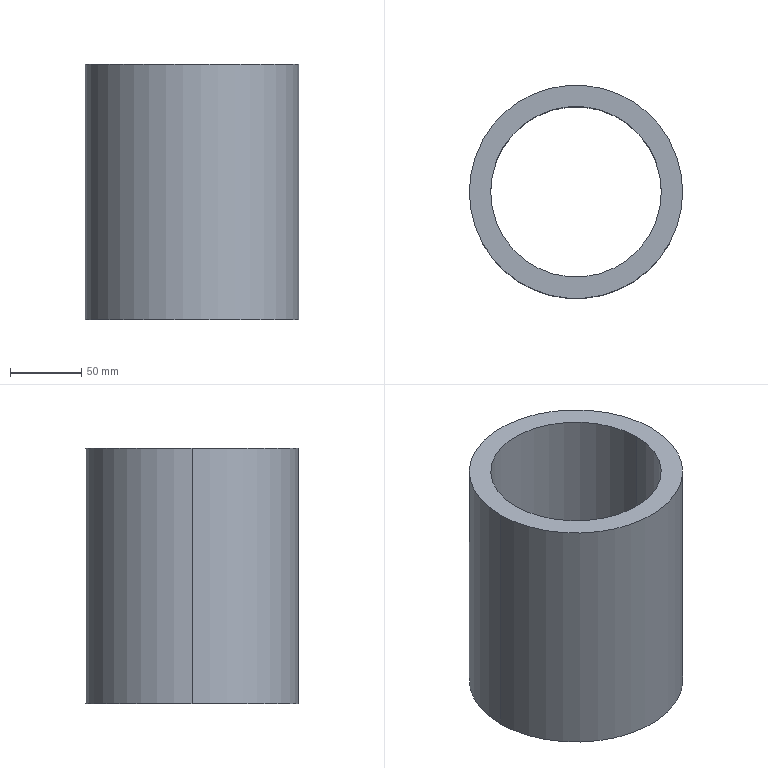Part | SolidWorks | features Extrusion 1 | 1 solid | 6 faces | box 150 x 150 x 180 mm | volume 1145111 mm3 | cylinder 4 | plane 2 | commonest cylinder face diameters 120 x2 150 x2
STEP:
#1=CARTESIAN_POINT('',(-60.,0.,180.));
#2=VERTEX_POINT('',#1);
#3=CARTESIAN_POINT('',(60.,0.,180.));
#4=VERTEX_POINT('',#3);
#5=CARTESIAN_POINT('',(0.,0.,180.));
#6=DIRECTION('',(0.,0.,1.));
#7=DIRECTION('',(1.,0.,0.));
#8=AXIS2_PLACEMENT_3D('',#5,#6,#7);
#9=CIRCLE('',#8,60.);
#10=EDGE_CURVE('',#2,#4,#9,.T.);
#11=ORIENTED_EDGE('',*,*,#10,.T.);
#12=CARTESIAN_POINT('',(60.,0.,0.));
#13=VERTEX_POINT('',#12);
#14=CARTESIAN_POINT('',(60.,0.,180.));
#15=DIRECTION('',(0.,0.,-1.));
#16=VECTOR('',#15,1000.);
#17=LINE('',#14,#16);
#18=EDGE_CURVE('',#4,#13,#17,.T.);
#19=ORIENTED_EDGE('',*,*,#18,.T.);
#20=CARTESIAN_POINT('',(-60.,0.,0.));
#21=VERTEX_POINT('',#20);
#22=CARTESIAN_POINT('',(0.,0.,0.));
#23=DIRECTION('',(0.,0.,1.));
#24=DIRECTION('',(1.,0.,0.));
#25=AXIS2_PLACEMENT_3D('',#22,#23,#24);
#26=CIRCLE('',#25,60.);
#27=EDGE_CURVE('',#21,#13,#26,.T.);
#28=ORIENTED_EDGE('',*,*,#27,.F.);
#29=CARTESIAN_POINT('',(-60.,0.,180.));
#30=DIRECTION('',(0.,0.,-1.));
#31=VECTOR('',#30,1000.);
#32=LINE('',#29,#31);
#33=EDGE_CURVE('',#2,#21,#32,.T.);
#34=ORIENTED_EDGE('',*,*,#33,.F.);
#35=EDGE_LOOP('',(#11,#19,#28,#34));
#36=FACE_OUTER_BOUND('',#35,.T.);
#37=CARTESIAN_POINT('',(0.,0.,180.));
#38=DIRECTION('',(0.,0.,-1.));
#39=DIRECTION('',(-1.,0.,0.));
#40=AXIS2_PLACEMENT_3D('',#37,#38,#39);
#41=CYLINDRICAL_SURFACE('',#40,60.);
#42=ADVANCED_FACE('',(#36),#41,.F.);
#43=CARTESIAN_POINT('',(75.,0.,180.));
#44=VERTEX_POINT('',#43);
#45=CARTESIAN_POINT('',(-75.,0.,180.));
#46=VERTEX_POINT('',#45);
#47=CARTESIAN_POINT('',(0.,0.,180.));
#48=DIRECTION('',(0.,0.,1.));
#49=DIRECTION('',(1.,0.,0.));
#50=AXIS2_PLACEMENT_3D('',#47,#48,#49);
#51=CIRCLE('',#50,75.);
#52=EDGE_CURVE('',#44,#46,#51,.T.);
#53=ORIENTED_EDGE('',*,*,#52,.F.);
#54=CARTESIAN_POINT('',(75.,0.,0.));
#55=VERTEX_POINT('',#54);
#56=CARTESIAN_POINT('',(75.,0.,180.));
#57=DIRECTION('',(0.,0.,-1.));
#58=VECTOR('',#57,1000.);
#59=LINE('',#56,#58);
#60=EDGE_CURVE('',#44,#55,#59,.T.);
#61=ORIENTED_EDGE('',*,*,#60,.T.);
#62=CARTESIAN_POINT('',(-75.,0.,0.));
#63=VERTEX_POINT('',#62);
#64=CARTESIAN_POINT('',(0.,0.,0.));
#65=DIRECTION('',(0.,0.,1.));
#66=DIRECTION('',(1.,0.,0.));
#67=AXIS2_PLACEMENT_3D('',#64,#65,#66);
#68=CIRCLE('',#67,75.);
#69=EDGE_CURVE('',#55,#63,#68,.T.);
#70=ORIENTED_EDGE('',*,*,#69,.T.);
#71=CARTESIAN_POINT('',(-75.,0.,180.));
#72=DIRECTION('',(0.,0.,-1.));
#73=VECTOR('',#72,1000.);
#74=LINE('',#71,#73);
#75=EDGE_CURVE('',#46,#63,#74,.T.);
#76=ORIENTED_EDGE('',*,*,#75,.F.);
#77=EDGE_LOOP('',(#53,#61,#70,#76));
#78=FACE_OUTER_BOUND('',#77,.T.);
#79=CARTESIAN_POINT('',(0.,0.,180.));
#80=DIRECTION('',(0.,0.,-1.));
#81=DIRECTION('',(-1.,0.,0.));
#82=AXIS2_PLACEMENT_3D('',#79,#80,#81);
#83=CYLINDRICAL_SURFACE('',#82,75.);
#84=ADVANCED_FACE('',(#78),#83,.T.);
#85=CARTESIAN_POINT('',(0.,0.,180.));
#86=DIRECTION('',(0.,0.,1.));
#87=DIRECTION('',(1.,0.,0.));
#88=AXIS2_PLACEMENT_3D('',#85,#86,#87);
#89=CIRCLE('',#88,75.);
#90=EDGE_CURVE('',#46,#44,#89,.T.);
#91=ORIENTED_EDGE('',*,*,#90,.T.);
#92=ORIENTED_EDGE('',*,*,#52,.T.);
#93=EDGE_LOOP('',(#91,#92));
#94=FACE_OUTER_BOUND('',#93,.T.);
#95=ORIENTED_EDGE('',*,*,#10,.F.);
#96=CARTESIAN_POINT('',(0.,0.,180.));
#97=DIRECTION('',(0.,0.,1.));
#98=DIRECTION('',(1.,0.,0.));
#99=AXIS2_PLACEMENT_3D('',#96,#97,#98);
#100=CIRCLE('',#99,60.);
#101=EDGE_CURVE('',#4,#2,#100,.T.);
#102=ORIENTED_EDGE('',*,*,#101,.F.);
#103=EDGE_LOOP('',(#95,#102));
#104=FACE_BOUND('',#103,.T.);
#105=CARTESIAN_POINT('',(0.,0.,180.));
#106=DIRECTION('',(0.,0.,1.));
#107=DIRECTION('',(1.,0.,0.));
#108=AXIS2_PLACEMENT_3D('',#105,#106,#107);
#109=PLANE('',#108);
#110=ADVANCED_FACE('',(#94,#104),#109,.T.);
#111=CARTESIAN_POINT('',(0.,0.,0.));
#112=DIRECTION('',(0.,0.,1.));
#113=DIRECTION('',(1.,0.,0.));
#114=AXIS2_PLACEMENT_3D('',#111,#112,#113);
#115=CIRCLE('',#114,75.);
#116=EDGE_CURVE('',#63,#55,#115,.T.);
#117=ORIENTED_EDGE('',*,*,#116,.F.);
#118=ORIENTED_EDGE('',*,*,#69,.F.);
#119=EDGE_LOOP('',(#117,#118));
#120=FACE_OUTER_BOUND('',#119,.T.);
#121=ORIENTED_EDGE('',*,*,#27,.T.);
#122=CARTESIAN_POINT('',(0.,0.,0.));
#123=DIRECTION('',(0.,0.,1.));
#124=DIRECTION('',(1.,0.,0.));
#125=AXIS2_PLACEMENT_3D('',#122,#123,#124);
#126=CIRCLE('',#125,60.);
#127=EDGE_CURVE('',#13,#21,#126,.T.);
#128=ORIENTED_EDGE('',*,*,#127,.T.);
#129=EDGE_LOOP('',(#121,#128));
#130=FACE_BOUND('',#129,.T.);
#131=CARTESIAN_POINT('',(0.,0.,0.));
#132=DIRECTION('',(0.,0.,1.));
#133=DIRECTION('',(1.,0.,0.));
#134=AXIS2_PLACEMENT_3D('',#131,#132,#133);
#135=PLANE('',#134);
#136=ADVANCED_FACE('',(#120,#130),#135,.F.);
#137=ORIENTED_EDGE('',*,*,#60,.F.);
#138=ORIENTED_EDGE('',*,*,#90,.F.);
#139=ORIENTED_EDGE('',*,*,#75,.T.);
#140=ORIENTED_EDGE('',*,*,#116,.T.);
#141=EDGE_LOOP('',(#137,#138,#139,#140));
#142=FACE_OUTER_BOUND('',#141,.T.);
#143=CARTESIAN_POINT('',(0.,0.,180.));
#144=DIRECTION('',(0.,0.,-1.));
#145=DIRECTION('',(-1.,0.,0.));
#146=AXIS2_PLACEMENT_3D('',#143,#144,#145);
#147=CYLINDRICAL_SURFACE('',#146,75.);
#148=ADVANCED_FACE('',(#142),#147,.T.);
#149=ORIENTED_EDGE('',*,*,#18,.F.);
#150=ORIENTED_EDGE('',*,*,#101,.T.);
#151=ORIENTED_EDGE('',*,*,#33,.T.);
#152=ORIENTED_EDGE('',*,*,#127,.F.);
#153=EDGE_LOOP('',(#149,#150,#151,#152));
#154=FACE_OUTER_BOUND('',#153,.T.);
#155=CARTESIAN_POINT('',(0.,0.,180.));
#156=DIRECTION('',(0.,0.,-1.));
#157=DIRECTION('',(-1.,0.,0.));
#158=AXIS2_PLACEMENT_3D('',#155,#156,#157);
#159=CYLINDRICAL_SURFACE('',#158,60.);
#160=ADVANCED_FACE('',(#154),#159,.F.);
#161=CLOSED_SHELL('',(#42,#84,#110,#136,#148,#160));
#162=MANIFOLD_SOLID_BREP('',#161);
#163=CARTESIAN_POINT('',(0.,0.,0.));
#164=DIRECTION('',(0.,0.,1.));
#165=DIRECTION('',(1.,0.,0.));
#166=AXIS2_PLACEMENT_3D('',#163,#164,#165);
#167=(LENGTH_UNIT()NAMED_UNIT(*)SI_UNIT(.MILLI.,.METRE.));
#168=UNCERTAINTY_MEASURE_WITH_UNIT(LENGTH_MEASURE(0.00001),#167,'','');
#169=(NAMED_UNIT(*)PLANE_ANGLE_UNIT()SI_UNIT($,.RADIAN.));
#170=(NAMED_UNIT(*)SI_UNIT($,.STERADIAN.)SOLID_ANGLE_UNIT());
#171=(GEOMETRIC_REPRESENTATION_CONTEXT(3)GLOBAL_UNCERTAINTY_ASSIGNED_CONTEXT((#168))GLOBAL_UNIT_ASSIGNED_CONTEXT((#167,#169,#170))REPRESENTATION_CONTEXT('',''));
#172=ADVANCED_BREP_SHAPE_REPRESENTATION('',(#162,#166),#171);